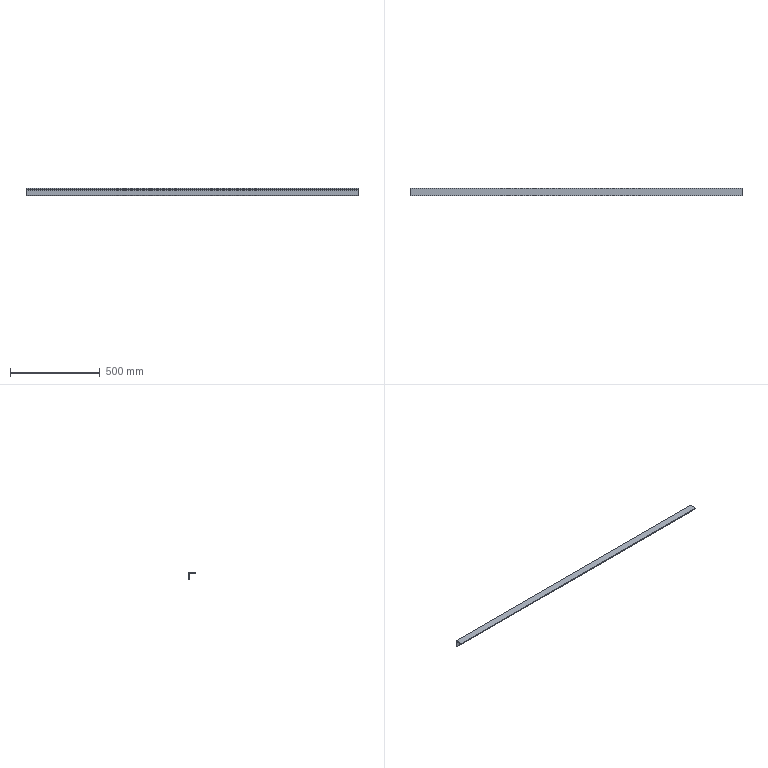Part | STEP file | Produce dryer frame-10_Default<As Machined> | 1 solid | 11 faces | box 1850 x 40 x 40 mm | volume 702264 mm3 | plane 8 | cylinder 3 | commonest cylinder face diameters 2.667 x2 10 x1
STEP:
#1=CARTESIAN_POINT('',(0.,-3.667,-40.));
#2=VERTEX_POINT('',#1);
#3=CARTESIAN_POINT('',(0.,0.,-40.));
#4=VERTEX_POINT('',#3);
#5=CARTESIAN_POINT('',(0.,0.,-40.));
#6=DIRECTION('',(0.,1.,0.));
#7=VECTOR('',#6,1000.);
#8=LINE('',#5,#7);
#9=EDGE_CURVE('',#2,#4,#8,.T.);
#10=ORIENTED_EDGE('',*,*,#9,.T.);
#11=CARTESIAN_POINT('',(1850.,0.,-40.));
#12=VERTEX_POINT('',#11);
#13=CARTESIAN_POINT('',(1850.,0.,-40.));
#14=DIRECTION('',(-1.,0.,0.));
#15=VECTOR('',#14,1000.);
#16=LINE('',#13,#15);
#17=EDGE_CURVE('',#12,#4,#16,.T.);
#18=ORIENTED_EDGE('',*,*,#17,.F.);
#19=CARTESIAN_POINT('',(1850.,-3.667,-40.));
#20=VERTEX_POINT('',#19);
#21=CARTESIAN_POINT('',(1850.,0.,-40.));
#22=DIRECTION('',(0.,1.,0.));
#23=VECTOR('',#22,1000.);
#24=LINE('',#21,#23);
#25=EDGE_CURVE('',#20,#12,#24,.T.);
#26=ORIENTED_EDGE('',*,*,#25,.F.);
#27=CARTESIAN_POINT('',(1850.,-3.667,-40.));
#28=DIRECTION('',(-1.,0.,0.));
#29=VECTOR('',#28,1000.);
#30=LINE('',#27,#29);
#31=EDGE_CURVE('',#20,#2,#30,.T.);
#32=ORIENTED_EDGE('',*,*,#31,.T.);
#33=EDGE_LOOP('',(#10,#18,#26,#32));
#34=FACE_OUTER_BOUND('',#33,.T.);
#35=CARTESIAN_POINT('',(1850.,0.,-40.));
#36=DIRECTION('',(0.,0.,1.));
#37=DIRECTION('',(0.,-1.,0.));
#38=AXIS2_PLACEMENT_3D('',#35,#36,#37);
#39=PLANE('',#38);
#40=ADVANCED_FACE('',(#34),#39,.F.);
#41=CARTESIAN_POINT('',(0.,0.,0.));
#42=VERTEX_POINT('',#41);
#43=CARTESIAN_POINT('',(0.,0.,-40.));
#44=DIRECTION('',(0.,0.,1.));
#45=VECTOR('',#44,1000.);
#46=LINE('',#43,#45);
#47=EDGE_CURVE('',#4,#42,#46,.T.);
#48=ORIENTED_EDGE('',*,*,#47,.T.);
#49=CARTESIAN_POINT('',(1850.,0.,0.));
#50=VERTEX_POINT('',#49);
#51=CARTESIAN_POINT('',(1850.,0.,0.));
#52=DIRECTION('',(-1.,0.,0.));
#53=VECTOR('',#52,1000.);
#54=LINE('',#51,#53);
#55=EDGE_CURVE('',#50,#42,#54,.T.);
#56=ORIENTED_EDGE('',*,*,#55,.F.);
#57=CARTESIAN_POINT('',(1850.,0.,-40.));
#58=DIRECTION('',(0.,0.,1.));
#59=VECTOR('',#58,1000.);
#60=LINE('',#57,#59);
#61=EDGE_CURVE('',#12,#50,#60,.T.);
#62=ORIENTED_EDGE('',*,*,#61,.F.);
#63=ORIENTED_EDGE('',*,*,#17,.T.);
#64=EDGE_LOOP('',(#48,#56,#62,#63));
#65=FACE_OUTER_BOUND('',#64,.T.);
#66=CARTESIAN_POINT('',(1850.,0.,-40.));
#67=DIRECTION('',(0.,-1.,0.));
#68=DIRECTION('',(0.,0.,-1.));
#69=AXIS2_PLACEMENT_3D('',#66,#67,#68);
#70=PLANE('',#69);
#71=ADVANCED_FACE('',(#65),#70,.F.);
#72=CARTESIAN_POINT('',(0.,-40.,0.));
#73=VERTEX_POINT('',#72);
#74=CARTESIAN_POINT('',(0.,0.,0.));
#75=DIRECTION('',(0.,-1.,0.));
#76=VECTOR('',#75,1000.);
#77=LINE('',#74,#76);
#78=EDGE_CURVE('',#42,#73,#77,.T.);
#79=ORIENTED_EDGE('',*,*,#78,.T.);
#80=CARTESIAN_POINT('',(1850.,-40.,0.));
#81=VERTEX_POINT('',#80);
#82=CARTESIAN_POINT('',(1850.,-40.,0.));
#83=DIRECTION('',(-1.,0.,0.));
#84=VECTOR('',#83,1000.);
#85=LINE('',#82,#84);
#86=EDGE_CURVE('',#81,#73,#85,.T.);
#87=ORIENTED_EDGE('',*,*,#86,.F.);
#88=CARTESIAN_POINT('',(1850.,0.,0.));
#89=DIRECTION('',(0.,-1.,0.));
#90=VECTOR('',#89,1000.);
#91=LINE('',#88,#90);
#92=EDGE_CURVE('',#50,#81,#91,.T.);
#93=ORIENTED_EDGE('',*,*,#92,.F.);
#94=ORIENTED_EDGE('',*,*,#55,.T.);
#95=EDGE_LOOP('',(#79,#87,#93,#94));
#96=FACE_OUTER_BOUND('',#95,.T.);
#97=CARTESIAN_POINT('',(1850.,0.,0.));
#98=DIRECTION('',(0.,0.,-1.));
#99=DIRECTION('',(0.,1.,0.));
#100=AXIS2_PLACEMENT_3D('',#97,#98,#99);
#101=PLANE('',#100);
#102=ADVANCED_FACE('',(#96),#101,.F.);
#103=CARTESIAN_POINT('',(0.,-40.,-3.667));
#104=VERTEX_POINT('',#103);
#105=CARTESIAN_POINT('',(0.,-40.,0.));
#106=DIRECTION('',(0.,0.,-1.));
#107=VECTOR('',#106,1000.);
#108=LINE('',#105,#107);
#109=EDGE_CURVE('',#73,#104,#108,.T.);
#110=ORIENTED_EDGE('',*,*,#109,.T.);
#111=CARTESIAN_POINT('',(1850.,-40.,-3.667));
#112=VERTEX_POINT('',#111);
#113=CARTESIAN_POINT('',(1850.,-40.,-3.667));
#114=DIRECTION('',(-1.,0.,0.));
#115=VECTOR('',#114,1000.);
#116=LINE('',#113,#115);
#117=EDGE_CURVE('',#112,#104,#116,.T.);
#118=ORIENTED_EDGE('',*,*,#117,.F.);
#119=CARTESIAN_POINT('',(1850.,-40.,0.));
#120=DIRECTION('',(0.,0.,-1.));
#121=VECTOR('',#120,1000.);
#122=LINE('',#119,#121);
#123=EDGE_CURVE('',#81,#112,#122,.T.);
#124=ORIENTED_EDGE('',*,*,#123,.F.);
#125=ORIENTED_EDGE('',*,*,#86,.T.);
#126=EDGE_LOOP('',(#110,#118,#124,#125));
#127=FACE_OUTER_BOUND('',#126,.T.);
#128=CARTESIAN_POINT('',(1850.,-40.,0.));
#129=DIRECTION('',(0.,1.,0.));
#130=DIRECTION('',(0.,0.,1.));
#131=AXIS2_PLACEMENT_3D('',#128,#129,#130);
#132=PLANE('',#131);
#133=ADVANCED_FACE('',(#127),#132,.F.);
#134=CARTESIAN_POINT('',(0.,-38.667,-5.));
#135=VERTEX_POINT('',#134);
#136=CARTESIAN_POINT('',(0.,-38.667,-3.667));
#137=DIRECTION('',(1.,0.,0.));
#138=DIRECTION('',(0.,0.,-1.));
#139=AXIS2_PLACEMENT_3D('',#136,#137,#138);
#140=CIRCLE('',#139,1.333);
#141=EDGE_CURVE('',#104,#135,#140,.T.);
#142=ORIENTED_EDGE('',*,*,#141,.T.);
#143=CARTESIAN_POINT('',(1850.,-38.667,-5.));
#144=VERTEX_POINT('',#143);
#145=CARTESIAN_POINT('',(1850.,-38.667,-5.));
#146=DIRECTION('',(-1.,0.,0.));
#147=VECTOR('',#146,1000.);
#148=LINE('',#145,#147);
#149=EDGE_CURVE('',#144,#135,#148,.T.);
#150=ORIENTED_EDGE('',*,*,#149,.F.);
#151=CARTESIAN_POINT('',(1850.,-38.667,-3.667));
#152=DIRECTION('',(1.,0.,0.));
#153=DIRECTION('',(0.,0.,-1.));
#154=AXIS2_PLACEMENT_3D('',#151,#152,#153);
#155=CIRCLE('',#154,1.333);
#156=EDGE_CURVE('',#112,#144,#155,.T.);
#157=ORIENTED_EDGE('',*,*,#156,.F.);
#158=ORIENTED_EDGE('',*,*,#117,.T.);
#159=EDGE_LOOP('',(#142,#150,#157,#158));
#160=FACE_OUTER_BOUND('',#159,.T.);
#161=CARTESIAN_POINT('',(1850.,-38.667,-3.667));
#162=DIRECTION('',(-1.,0.,0.));
#163=DIRECTION('',(0.,0.,1.));
#164=AXIS2_PLACEMENT_3D('',#161,#162,#163);
#165=CYLINDRICAL_SURFACE('',#164,1.333);
#166=ADVANCED_FACE('',(#160),#165,.T.);
#167=CARTESIAN_POINT('',(0.,-10.,-5.));
#168=VERTEX_POINT('',#167);
#169=CARTESIAN_POINT('',(0.,-10.,-5.));
#170=DIRECTION('',(0.,1.,0.));
#171=VECTOR('',#170,1000.);
#172=LINE('',#169,#171);
#173=EDGE_CURVE('',#135,#168,#172,.T.);
#174=ORIENTED_EDGE('',*,*,#173,.T.);
#175=CARTESIAN_POINT('',(1850.,-10.,-5.));
#176=VERTEX_POINT('',#175);
#177=CARTESIAN_POINT('',(1850.,-10.,-5.));
#178=DIRECTION('',(-1.,0.,0.));
#179=VECTOR('',#178,1000.);
#180=LINE('',#177,#179);
#181=EDGE_CURVE('',#176,#168,#180,.T.);
#182=ORIENTED_EDGE('',*,*,#181,.F.);
#183=CARTESIAN_POINT('',(1850.,-10.,-5.));
#184=DIRECTION('',(0.,1.,0.));
#185=VECTOR('',#184,1000.);
#186=LINE('',#183,#185);
#187=EDGE_CURVE('',#144,#176,#186,.T.);
#188=ORIENTED_EDGE('',*,*,#187,.F.);
#189=ORIENTED_EDGE('',*,*,#149,.T.);
#190=EDGE_LOOP('',(#174,#182,#188,#189));
#191=FACE_OUTER_BOUND('',#190,.T.);
#192=CARTESIAN_POINT('',(1850.,-10.,-5.));
#193=DIRECTION('',(0.,0.,1.));
#194=DIRECTION('',(0.,-1.,0.));
#195=AXIS2_PLACEMENT_3D('',#192,#193,#194);
#196=PLANE('',#195);
#197=ADVANCED_FACE('',(#191),#196,.F.);
#198=CARTESIAN_POINT('',(0.,-5.,-10.));
#199=VERTEX_POINT('',#198);
#200=CARTESIAN_POINT('',(0.,-10.,-10.));
#201=DIRECTION('',(-1.,0.,0.));
#202=DIRECTION('',(0.,0.,-1.));
#203=AXIS2_PLACEMENT_3D('',#200,#201,#202);
#204=CIRCLE('',#203,5.);
#205=EDGE_CURVE('',#168,#199,#204,.T.);
#206=ORIENTED_EDGE('',*,*,#205,.T.);
#207=CARTESIAN_POINT('',(1850.,-5.,-10.));
#208=VERTEX_POINT('',#207);
#209=CARTESIAN_POINT('',(1850.,-5.,-10.));
#210=DIRECTION('',(-1.,0.,0.));
#211=VECTOR('',#210,1000.);
#212=LINE('',#209,#211);
#213=EDGE_CURVE('',#208,#199,#212,.T.);
#214=ORIENTED_EDGE('',*,*,#213,.F.);
#215=CARTESIAN_POINT('',(1850.,-10.,-10.));
#216=DIRECTION('',(-1.,0.,0.));
#217=DIRECTION('',(0.,0.,-1.));
#218=AXIS2_PLACEMENT_3D('',#215,#216,#217);
#219=CIRCLE('',#218,5.);
#220=EDGE_CURVE('',#176,#208,#219,.T.);
#221=ORIENTED_EDGE('',*,*,#220,.F.);
#222=ORIENTED_EDGE('',*,*,#181,.T.);
#223=EDGE_LOOP('',(#206,#214,#221,#222));
#224=FACE_OUTER_BOUND('',#223,.T.);
#225=CARTESIAN_POINT('',(1850.,-10.,-10.));
#226=DIRECTION('',(-1.,0.,0.));
#227=DIRECTION('',(0.,0.,1.));
#228=AXIS2_PLACEMENT_3D('',#225,#226,#227);
#229=CYLINDRICAL_SURFACE('',#228,5.);
#230=ADVANCED_FACE('',(#224),#229,.F.);
#231=CARTESIAN_POINT('',(0.,-5.,-38.667));
#232=VERTEX_POINT('',#231);
#233=CARTESIAN_POINT('',(0.,-5.,-38.667));
#234=DIRECTION('',(0.,0.,-1.));
#235=VECTOR('',#234,1000.);
#236=LINE('',#233,#235);
#237=EDGE_CURVE('',#199,#232,#236,.T.);
#238=ORIENTED_EDGE('',*,*,#237,.T.);
#239=CARTESIAN_POINT('',(1850.,-5.,-38.667));
#240=VERTEX_POINT('',#239);
#241=CARTESIAN_POINT('',(1850.,-5.,-38.667));
#242=DIRECTION('',(-1.,0.,0.));
#243=VECTOR('',#242,1000.);
#244=LINE('',#241,#243);
#245=EDGE_CURVE('',#240,#232,#244,.T.);
#246=ORIENTED_EDGE('',*,*,#245,.F.);
#247=CARTESIAN_POINT('',(1850.,-5.,-38.667));
#248=DIRECTION('',(0.,0.,-1.));
#249=VECTOR('',#248,1000.);
#250=LINE('',#247,#249);
#251=EDGE_CURVE('',#208,#240,#250,.T.);
#252=ORIENTED_EDGE('',*,*,#251,.F.);
#253=ORIENTED_EDGE('',*,*,#213,.T.);
#254=EDGE_LOOP('',(#238,#246,#252,#253));
#255=FACE_OUTER_BOUND('',#254,.T.);
#256=CARTESIAN_POINT('',(1850.,-5.,-38.667));
#257=DIRECTION('',(0.,1.,0.));
#258=DIRECTION('',(0.,0.,1.));
#259=AXIS2_PLACEMENT_3D('',#256,#257,#258);
#260=PLANE('',#259);
#261=ADVANCED_FACE('',(#255),#260,.F.);
#262=CARTESIAN_POINT('',(0.,-3.667,-38.667));
#263=DIRECTION('',(1.,0.,0.));
#264=DIRECTION('',(0.,0.,1.));
#265=AXIS2_PLACEMENT_3D('',#262,#263,#264);
#266=CIRCLE('',#265,1.333);
#267=EDGE_CURVE('',#232,#2,#266,.T.);
#268=ORIENTED_EDGE('',*,*,#267,.T.);
#269=ORIENTED_EDGE('',*,*,#31,.F.);
#270=CARTESIAN_POINT('',(1850.,-3.667,-38.667));
#271=DIRECTION('',(1.,0.,0.));
#272=DIRECTION('',(0.,0.,1.));
#273=AXIS2_PLACEMENT_3D('',#270,#271,#272);
#274=CIRCLE('',#273,1.333);
#275=EDGE_CURVE('',#240,#20,#274,.T.);
#276=ORIENTED_EDGE('',*,*,#275,.F.);
#277=ORIENTED_EDGE('',*,*,#245,.T.);
#278=EDGE_LOOP('',(#268,#269,#276,#277));
#279=FACE_OUTER_BOUND('',#278,.T.);
#280=CARTESIAN_POINT('',(1850.,-3.667,-38.667));
#281=DIRECTION('',(-1.,0.,0.));
#282=DIRECTION('',(0.,0.,1.));
#283=AXIS2_PLACEMENT_3D('',#280,#281,#282);
#284=CYLINDRICAL_SURFACE('',#283,1.333);
#285=ADVANCED_FACE('',(#279),#284,.T.);
#286=ORIENTED_EDGE('',*,*,#25,.T.);
#287=ORIENTED_EDGE('',*,*,#61,.T.);
#288=ORIENTED_EDGE('',*,*,#92,.T.);
#289=ORIENTED_EDGE('',*,*,#123,.T.);
#290=ORIENTED_EDGE('',*,*,#156,.T.);
#291=ORIENTED_EDGE('',*,*,#187,.T.);
#292=ORIENTED_EDGE('',*,*,#220,.T.);
#293=ORIENTED_EDGE('',*,*,#251,.T.);
#294=ORIENTED_EDGE('',*,*,#275,.T.);
#295=EDGE_LOOP('',(#286,#287,#288,#289,#290,#291,#292,#293,#294));
#296=FACE_OUTER_BOUND('',#295,.T.);
#297=CARTESIAN_POINT('',(1850.,-3.667,-38.667));
#298=DIRECTION('',(-1.,0.,0.));
#299=DIRECTION('',(0.,0.,1.));
#300=AXIS2_PLACEMENT_3D('',#297,#298,#299);
#301=PLANE('',#300);
#302=ADVANCED_FACE('',(#296),#301,.F.);
#303=ORIENTED_EDGE('',*,*,#9,.F.);
#304=ORIENTED_EDGE('',*,*,#267,.F.);
#305=ORIENTED_EDGE('',*,*,#237,.F.);
#306=ORIENTED_EDGE('',*,*,#205,.F.);
#307=ORIENTED_EDGE('',*,*,#173,.F.);
#308=ORIENTED_EDGE('',*,*,#141,.F.);
#309=ORIENTED_EDGE('',*,*,#109,.F.);
#310=ORIENTED_EDGE('',*,*,#78,.F.);
#311=ORIENTED_EDGE('',*,*,#47,.F.);
#312=EDGE_LOOP('',(#303,#304,#305,#306,#307,#308,#309,#310,#311));
#313=FACE_OUTER_BOUND('',#312,.T.);
#314=CARTESIAN_POINT('',(0.,-3.667,-38.667));
#315=DIRECTION('',(-1.,0.,0.));
#316=DIRECTION('',(0.,0.,1.));
#317=AXIS2_PLACEMENT_3D('',#314,#315,#316);
#318=PLANE('',#317);
#319=ADVANCED_FACE('',(#313),#318,.T.);
#320=CLOSED_SHELL('',(#40,#71,#102,#133,#166,#197,#230,#261,#285,#302,#319));
#321=MANIFOLD_SOLID_BREP('',#320);
#322=CARTESIAN_POINT('',(0.,0.,0.));
#323=DIRECTION('',(0.,0.,1.));
#324=DIRECTION('',(1.,0.,0.));
#325=AXIS2_PLACEMENT_3D('',#322,#323,#324);
#326=(LENGTH_UNIT()NAMED_UNIT(*)SI_UNIT(.MILLI.,.METRE.));
#327=UNCERTAINTY_MEASURE_WITH_UNIT(LENGTH_MEASURE(0.00001),#326,'','');
#328=(NAMED_UNIT(*)PLANE_ANGLE_UNIT()SI_UNIT($,.RADIAN.));
#329=(NAMED_UNIT(*)SI_UNIT($,.STERADIAN.)SOLID_ANGLE_UNIT());
#330=(GEOMETRIC_REPRESENTATION_CONTEXT(3)GLOBAL_UNCERTAINTY_ASSIGNED_CONTEXT((#327))GLOBAL_UNIT_ASSIGNED_CONTEXT((#326,#328,#329))REPRESENTATION_CONTEXT('',''));
#331=ADVANCED_BREP_SHAPE_REPRESENTATION('',(#321,#325),#330);